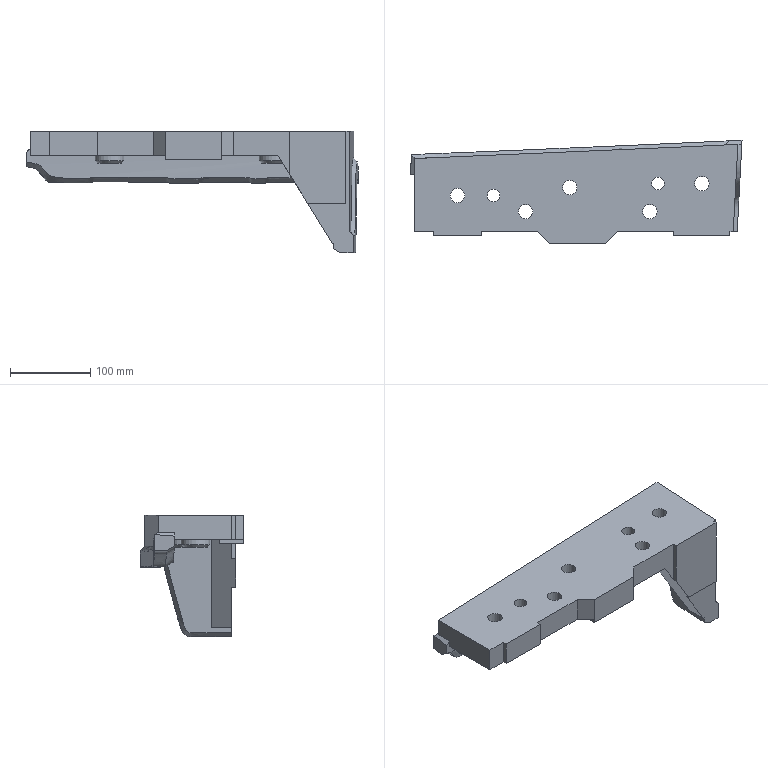Part | NX | features solid 2 | 1 solid | 68 faces | box 414.214 x 129.147 x 152.075 mm | volume 1843060 mm3 | plane 35 | spline 17 | cylinder 14 | cone 2 | commonest cylinder face diameters 18 x5 26 x5 16 x2 36 x2